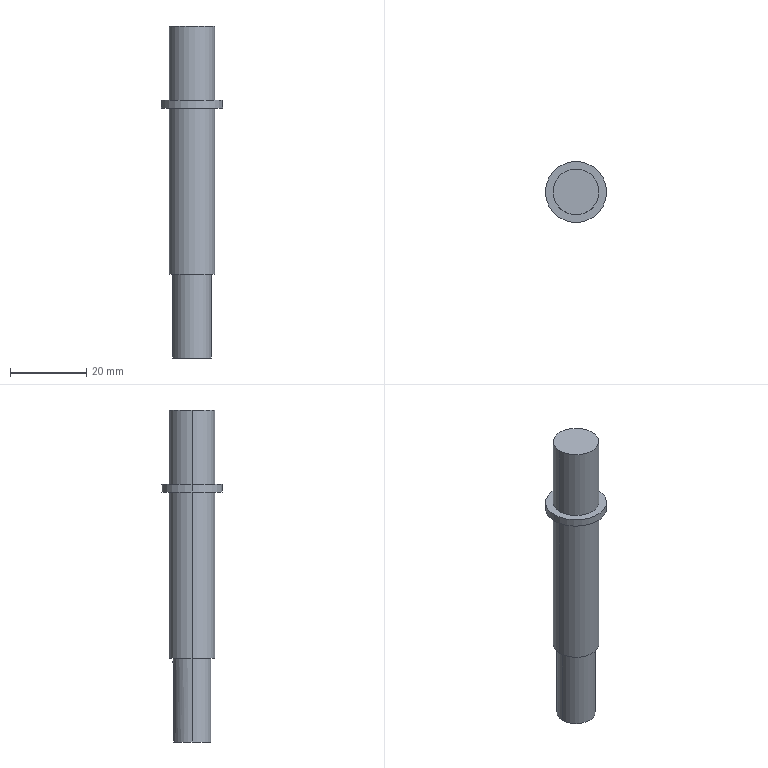Part | SolidWorks | features ICE 2, Extrusion 1, HoleWzd 1, Revolution 1 | 1 solid | 21 faces | box 16 x 16 x 87 mm | volume 9059 mm3 | cylinder 11 | plane 8 | cone 2 | commonest cylinder face diameters 12 x4 3.3 x2 10 x2 16 x2 3 x1
STEP:
#1=CARTESIAN_POINT('',(1.65,0.,-11.9));
#2=VERTEX_POINT('',#1);
#3=CARTESIAN_POINT('',(-1.65,0.,-11.9));
#4=VERTEX_POINT('',#3);
#5=CARTESIAN_POINT('',(0.,0.,-11.9));
#6=DIRECTION('',(0.,0.,-1.));
#7=DIRECTION('',(-1.,0.,0.));
#8=AXIS2_PLACEMENT_3D('',#5,#6,#7);
#9=CIRCLE('',#8,1.65);
#10=EDGE_CURVE('',#2,#4,#9,.T.);
#11=ORIENTED_EDGE('',*,*,#10,.F.);
#12=CARTESIAN_POINT('',(1.65,0.,-22.));
#13=VERTEX_POINT('',#12);
#14=CARTESIAN_POINT('',(1.65,0.,-22.));
#15=DIRECTION('',(0.,0.,-1.));
#16=VECTOR('',#15,1000.);
#17=LINE('',#14,#16);
#18=EDGE_CURVE('',#2,#13,#17,.T.);
#19=ORIENTED_EDGE('',*,*,#18,.T.);
#20=CARTESIAN_POINT('',(-1.65,0.,-22.));
#21=VERTEX_POINT('',#20);
#22=CARTESIAN_POINT('',(0.,0.,-22.));
#23=DIRECTION('',(0.,0.,-1.));
#24=DIRECTION('',(-1.,0.,0.));
#25=AXIS2_PLACEMENT_3D('',#22,#23,#24);
#26=CIRCLE('',#25,1.65);
#27=EDGE_CURVE('',#13,#21,#26,.T.);
#28=ORIENTED_EDGE('',*,*,#27,.T.);
#29=CARTESIAN_POINT('',(-1.65,0.,-22.));
#30=DIRECTION('',(0.,0.,-1.));
#31=VECTOR('',#30,1000.);
#32=LINE('',#29,#31);
#33=EDGE_CURVE('',#4,#21,#32,.T.);
#34=ORIENTED_EDGE('',*,*,#33,.F.);
#35=EDGE_LOOP('',(#11,#19,#28,#34));
#36=FACE_OUTER_BOUND('',#35,.T.);
#37=CARTESIAN_POINT('',(0.,0.,-22.));
#38=DIRECTION('',(0.,0.,-1.));
#39=DIRECTION('',(-1.,0.,0.));
#40=AXIS2_PLACEMENT_3D('',#37,#38,#39);
#41=CYLINDRICAL_SURFACE('',#40,1.65);
#42=ADVANCED_FACE('',(#36),#41,.F.);
#43=CARTESIAN_POINT('',(0.,0.,-10.909));
#44=VERTEX_POINT('',#43);
#45=CARTESIAN_POINT('',(-1.65,0.,-11.9));
#46=DIRECTION('',(-0.8572,0.,-0.515));
#47=VECTOR('',#46,1000.);
#48=LINE('',#45,#47);
#49=EDGE_CURVE('',#44,#4,#48,.T.);
#50=ORIENTED_EDGE('',*,*,#49,.F.);
#51=CARTESIAN_POINT('',(1.65,0.,-11.9));
#52=DIRECTION('',(0.8572,0.,-0.515));
#53=VECTOR('',#52,1000.);
#54=LINE('',#51,#53);
#55=EDGE_CURVE('',#44,#2,#54,.T.);
#56=ORIENTED_EDGE('',*,*,#55,.T.);
#57=ORIENTED_EDGE('',*,*,#10,.T.);
#58=EDGE_LOOP('',(#50,#56,#57));
#59=FACE_OUTER_BOUND('',#58,.T.);
#60=CARTESIAN_POINT('',(0.,0.,-11.9));
#61=DIRECTION('',(0.,0.,-1.));
#62=DIRECTION('',(-1.,0.,0.));
#63=AXIS2_PLACEMENT_3D('',#60,#61,#62);
#64=CONICAL_SURFACE('',#63,1.65,1.03);
#65=ADVANCED_FACE('',(#59),#64,.F.);
#66=CARTESIAN_POINT('',(6.,0.,65.));
#67=VERTEX_POINT('',#66);
#68=CARTESIAN_POINT('',(-6.,0.,65.));
#69=VERTEX_POINT('',#68);
#70=CARTESIAN_POINT('',(0.,0.,65.));
#71=DIRECTION('',(0.,0.,1.));
#72=DIRECTION('',(1.,0.,0.));
#73=AXIS2_PLACEMENT_3D('',#70,#71,#72);
#74=CIRCLE('',#73,6.);
#75=EDGE_CURVE('',#67,#69,#74,.T.);
#76=ORIENTED_EDGE('',*,*,#75,.F.);
#77=CARTESIAN_POINT('',(6.,0.,45.5));
#78=VERTEX_POINT('',#77);
#79=CARTESIAN_POINT('',(6.,0.,65.));
#80=DIRECTION('',(0.,0.,-1.));
#81=VECTOR('',#80,1000.);
#82=LINE('',#79,#81);
#83=EDGE_CURVE('',#67,#78,#82,.T.);
#84=ORIENTED_EDGE('',*,*,#83,.T.);
#85=CARTESIAN_POINT('',(-6.,0.,45.5));
#86=VERTEX_POINT('',#85);
#87=CARTESIAN_POINT('',(0.,0.,45.5));
#88=DIRECTION('',(0.,0.,-1.));
#89=DIRECTION('',(-1.,0.,0.));
#90=AXIS2_PLACEMENT_3D('',#87,#88,#89);
#91=CIRCLE('',#90,6.);
#92=EDGE_CURVE('',#86,#78,#91,.T.);
#93=ORIENTED_EDGE('',*,*,#92,.F.);
#94=CARTESIAN_POINT('',(-6.,0.,65.));
#95=DIRECTION('',(0.,0.,-1.));
#96=VECTOR('',#95,1000.);
#97=LINE('',#94,#96);
#98=EDGE_CURVE('',#69,#86,#97,.T.);
#99=ORIENTED_EDGE('',*,*,#98,.F.);
#100=EDGE_LOOP('',(#76,#84,#93,#99));
#101=FACE_OUTER_BOUND('',#100,.T.);
#102=CARTESIAN_POINT('',(0.,0.,65.));
#103=DIRECTION('',(0.,0.,-1.));
#104=DIRECTION('',(-1.,0.,0.));
#105=AXIS2_PLACEMENT_3D('',#102,#103,#104);
#106=CYLINDRICAL_SURFACE('',#105,6.);
#107=ADVANCED_FACE('',(#101),#106,.T.);
#108=CARTESIAN_POINT('',(8.,0.,43.5));
#109=VERTEX_POINT('',#108);
#110=CARTESIAN_POINT('',(-8.,0.,43.5));
#111=VERTEX_POINT('',#110);
#112=CARTESIAN_POINT('',(0.,0.,43.5));
#113=DIRECTION('',(0.,0.,1.));
#114=DIRECTION('',(1.,0.,0.));
#115=AXIS2_PLACEMENT_3D('',#112,#113,#114);
#116=CIRCLE('',#115,8.);
#117=EDGE_CURVE('',#109,#111,#116,.T.);
#118=ORIENTED_EDGE('',*,*,#117,.T.);
#119=CARTESIAN_POINT('',(-8.,0.,45.5));
#120=VERTEX_POINT('',#119);
#121=CARTESIAN_POINT('',(-8.,0.,65.));
#122=DIRECTION('',(0.,0.,1.));
#123=VECTOR('',#122,1000.);
#124=LINE('',#121,#123);
#125=EDGE_CURVE('',#111,#120,#124,.T.);
#126=ORIENTED_EDGE('',*,*,#125,.T.);
#127=CARTESIAN_POINT('',(8.,0.,45.5));
#128=VERTEX_POINT('',#127);
#129=CARTESIAN_POINT('',(0.,0.,45.5));
#130=DIRECTION('',(0.,0.,1.));
#131=DIRECTION('',(1.,0.,0.));
#132=AXIS2_PLACEMENT_3D('',#129,#130,#131);
#133=CIRCLE('',#132,8.);
#134=EDGE_CURVE('',#128,#120,#133,.T.);
#135=ORIENTED_EDGE('',*,*,#134,.F.);
#136=CARTESIAN_POINT('',(8.,0.,65.));
#137=DIRECTION('',(0.,0.,1.));
#138=VECTOR('',#137,1000.);
#139=LINE('',#136,#138);
#140=EDGE_CURVE('',#109,#128,#139,.T.);
#141=ORIENTED_EDGE('',*,*,#140,.F.);
#142=EDGE_LOOP('',(#118,#126,#135,#141));
#143=FACE_OUTER_BOUND('',#142,.T.);
#144=CARTESIAN_POINT('',(0.,0.,65.));
#145=DIRECTION('',(0.,0.,1.));
#146=DIRECTION('',(1.,0.,0.));
#147=AXIS2_PLACEMENT_3D('',#144,#145,#146);
#148=CYLINDRICAL_SURFACE('',#147,8.);
#149=ADVANCED_FACE('',(#143),#148,.T.);
#150=CARTESIAN_POINT('',(-5.,0.,-22.));
#151=VERTEX_POINT('',#150);
#152=CARTESIAN_POINT('',(-1.5,4.77,-22.));
#153=VERTEX_POINT('',#152);
#154=CARTESIAN_POINT('',(0.,0.,-22.));
#155=DIRECTION('',(0.,0.,-1.));
#156=DIRECTION('',(-1.,0.,0.));
#157=AXIS2_PLACEMENT_3D('',#154,#155,#156);
#158=CIRCLE('',#157,5.);
#159=EDGE_CURVE('',#151,#153,#158,.T.);
#160=ORIENTED_EDGE('',*,*,#159,.F.);
#161=CARTESIAN_POINT('',(-5.,0.,0.));
#162=VERTEX_POINT('',#161);
#163=CARTESIAN_POINT('',(-5.,0.,-22.));
#164=DIRECTION('',(0.,0.,1.));
#165=VECTOR('',#164,1000.);
#166=LINE('',#163,#165);
#167=EDGE_CURVE('',#151,#162,#166,.T.);
#168=ORIENTED_EDGE('',*,*,#167,.T.);
#169=CARTESIAN_POINT('',(5.,0.,0.));
#170=VERTEX_POINT('',#169);
#171=CARTESIAN_POINT('',(0.,0.,0.));
#172=DIRECTION('',(0.,0.,-1.));
#173=DIRECTION('',(-1.,0.,0.));
#174=AXIS2_PLACEMENT_3D('',#171,#172,#173);
#175=CIRCLE('',#174,5.);
#176=EDGE_CURVE('',#162,#170,#175,.T.);
#177=ORIENTED_EDGE('',*,*,#176,.T.);
#178=CARTESIAN_POINT('',(5.,0.,-22.));
#179=VERTEX_POINT('',#178);
#180=CARTESIAN_POINT('',(5.,0.,-22.));
#181=DIRECTION('',(0.,0.,1.));
#182=VECTOR('',#181,1000.);
#183=LINE('',#180,#182);
#184=EDGE_CURVE('',#179,#170,#183,.T.);
#185=ORIENTED_EDGE('',*,*,#184,.F.);
#186=CARTESIAN_POINT('',(1.5,4.77,-22.));
#187=VERTEX_POINT('',#186);
#188=CARTESIAN_POINT('',(0.,0.,-22.));
#189=DIRECTION('',(0.,0.,-1.));
#190=DIRECTION('',(-1.,0.,0.));
#191=AXIS2_PLACEMENT_3D('',#188,#189,#190);
#192=CIRCLE('',#191,5.);
#193=EDGE_CURVE('',#187,#179,#192,.T.);
#194=ORIENTED_EDGE('',*,*,#193,.F.);
#195=CARTESIAN_POINT('',(1.5,4.77,-2.5));
#196=VERTEX_POINT('',#195);
#197=CARTESIAN_POINT('',(1.5,4.77,-22.));
#198=DIRECTION('',(0.,0.,1.));
#199=VECTOR('',#198,1000.);
#200=LINE('',#197,#199);
#201=EDGE_CURVE('',#187,#196,#200,.T.);
#202=ORIENTED_EDGE('',*,*,#201,.T.);
#203=CARTESIAN_POINT('',(-1.5,4.77,-2.5));
#204=VERTEX_POINT('',#203);
#205=CARTESIAN_POINT('',(1.5,4.77,-2.5));
#206=CARTESIAN_POINT('',(1.5,4.77,-2.4));
#207=CARTESIAN_POINT('',(1.49,4.773,-2.302));
#208=CARTESIAN_POINT('',(1.452,4.785,-2.11));
#209=CARTESIAN_POINT('',(1.423,4.794,-2.014));
#210=CARTESIAN_POINT('',(1.347,4.815,-1.833));
#211=CARTESIAN_POINT('',(1.301,4.828,-1.747));
#212=CARTESIAN_POINT('',(1.192,4.856,-1.585));
#213=CARTESIAN_POINT('',(1.129,4.871,-1.508));
#214=CARTESIAN_POINT('',(0.9233,4.916,-1.302));
#215=CARTESIAN_POINT('',(0.7569,4.946,-1.19));
#216=CARTESIAN_POINT('',(0.3965,4.988,-1.04));
#217=CARTESIAN_POINT('',(0.1984,5.,-1.));
#218=CARTESIAN_POINT('',(-0.09698,5.,-0.9999));
#219=CARTESIAN_POINT('',(-0.197,4.997,-1.01));
#220=CARTESIAN_POINT('',(-0.3898,4.986,-1.048));
#221=CARTESIAN_POINT('',(-0.4837,4.977,-1.077));
#222=CARTESIAN_POINT('',(-0.7572,4.946,-1.19));
#223=CARTESIAN_POINT('',(-0.9219,4.916,-1.301));
#224=CARTESIAN_POINT('',(-1.13,4.871,-1.508));
#225=CARTESIAN_POINT('',(-1.191,4.856,-1.583));
#226=CARTESIAN_POINT('',(-1.3,4.828,-1.745));
#227=CARTESIAN_POINT('',(-1.347,4.815,-1.833));
#228=CARTESIAN_POINT('',(-1.46,4.783,-2.104));
#229=CARTESIAN_POINT('',(-1.5,4.77,-2.301));
#230=CARTESIAN_POINT('',(-1.5,4.77,-2.5));
#231=B_SPLINE_CURVE_WITH_KNOTS('',3,(#205,#206,#207,#208,#209,#210,#211,#212,#213,#214,#215,#216,#217,#218,#219,#220,#221,#222,#223,#224,#225,#226,#227,#228,#229,#230),.UNSPECIFIED.,.F.,.F.,(4,2,2,2,2,2,2,2,2,2,2,2,4),(0.,0.0002947,0.0005894,0.0008841,0.001179,0.001768,0.002358,0.002652,0.002947,0.003536,0.003831,0.004126,0.004715),.UNSPECIFIED.);
#232=EDGE_CURVE('',#196,#204,#231,.T.);
#233=ORIENTED_EDGE('',*,*,#232,.T.);
#234=CARTESIAN_POINT('',(-1.5,4.77,-22.));
#235=DIRECTION('',(0.,0.,-1.));
#236=VECTOR('',#235,1000.);
#237=LINE('',#234,#236);
#238=EDGE_CURVE('',#204,#153,#237,.T.);
#239=ORIENTED_EDGE('',*,*,#238,.T.);
#240=EDGE_LOOP('',(#160,#168,#177,#185,#194,#202,#233,#239));
#241=FACE_OUTER_BOUND('',#240,.T.);
#242=CARTESIAN_POINT('',(0.,0.,-22.));
#243=DIRECTION('',(0.,0.,1.));
#244=DIRECTION('',(1.,0.,0.));
#245=AXIS2_PLACEMENT_3D('',#242,#243,#244);
#246=CYLINDRICAL_SURFACE('',#245,5.);
#247=ADVANCED_FACE('',(#241),#246,.T.);
#248=CARTESIAN_POINT('',(6.,0.,43.5));
#249=VERTEX_POINT('',#248);
#250=CARTESIAN_POINT('',(-6.,0.,43.5));
#251=VERTEX_POINT('',#250);
#252=CARTESIAN_POINT('',(0.,0.,43.5));
#253=DIRECTION('',(0.,0.,1.));
#254=DIRECTION('',(1.,0.,0.));
#255=AXIS2_PLACEMENT_3D('',#252,#253,#254);
#256=CIRCLE('',#255,6.);
#257=EDGE_CURVE('',#249,#251,#256,.T.);
#258=ORIENTED_EDGE('',*,*,#257,.F.);
#259=CARTESIAN_POINT('',(6.,0.,0.));
#260=VERTEX_POINT('',#259);
#261=CARTESIAN_POINT('',(6.,0.,65.));
#262=DIRECTION('',(0.,0.,-1.));
#263=VECTOR('',#262,1000.);
#264=LINE('',#261,#263);
#265=EDGE_CURVE('',#249,#260,#264,.T.);
#266=ORIENTED_EDGE('',*,*,#265,.T.);
#267=CARTESIAN_POINT('',(-6.,0.,0.));
#268=VERTEX_POINT('',#267);
#269=CARTESIAN_POINT('',(0.,0.,0.));
#270=DIRECTION('',(0.,0.,1.));
#271=DIRECTION('',(1.,0.,0.));
#272=AXIS2_PLACEMENT_3D('',#269,#270,#271);
#273=CIRCLE('',#272,6.);
#274=EDGE_CURVE('',#260,#268,#273,.T.);
#275=ORIENTED_EDGE('',*,*,#274,.T.);
#276=CARTESIAN_POINT('',(-6.,0.,65.));
#277=DIRECTION('',(0.,0.,-1.));
#278=VECTOR('',#277,1000.);
#279=LINE('',#276,#278);
#280=EDGE_CURVE('',#251,#268,#279,.T.);
#281=ORIENTED_EDGE('',*,*,#280,.F.);
#282=EDGE_LOOP('',(#258,#266,#275,#281));
#283=FACE_OUTER_BOUND('',#282,.T.);
#284=CARTESIAN_POINT('',(0.,0.,65.));
#285=DIRECTION('',(0.,0.,-1.));
#286=DIRECTION('',(-1.,0.,0.));
#287=AXIS2_PLACEMENT_3D('',#284,#285,#286);
#288=CYLINDRICAL_SURFACE('',#287,6.);
#289=ADVANCED_FACE('',(#283),#288,.T.);
#290=ORIENTED_EDGE('',*,*,#265,.F.);
#291=CARTESIAN_POINT('',(0.,0.,43.5));
#292=DIRECTION('',(0.,0.,1.));
#293=DIRECTION('',(1.,0.,0.));
#294=AXIS2_PLACEMENT_3D('',#291,#292,#293);
#295=CIRCLE('',#294,6.);
#296=EDGE_CURVE('',#251,#249,#295,.T.);
#297=ORIENTED_EDGE('',*,*,#296,.F.);
#298=ORIENTED_EDGE('',*,*,#280,.T.);
#299=CARTESIAN_POINT('',(0.,0.,0.));
#300=DIRECTION('',(0.,0.,1.));
#301=DIRECTION('',(1.,0.,0.));
#302=AXIS2_PLACEMENT_3D('',#299,#300,#301);
#303=CIRCLE('',#302,6.);
#304=EDGE_CURVE('',#268,#260,#303,.T.);
#305=ORIENTED_EDGE('',*,*,#304,.T.);
#306=EDGE_LOOP('',(#290,#297,#298,#305));
#307=FACE_OUTER_BOUND('',#306,.T.);
#308=CARTESIAN_POINT('',(0.,0.,65.));
#309=DIRECTION('',(0.,0.,-1.));
#310=DIRECTION('',(-1.,0.,0.));
#311=AXIS2_PLACEMENT_3D('',#308,#309,#310);
#312=CYLINDRICAL_SURFACE('',#311,6.);
#313=ADVANCED_FACE('',(#307),#312,.T.);
#314=CARTESIAN_POINT('',(0.,0.,0.));
#315=DIRECTION('',(0.,0.,-1.));
#316=DIRECTION('',(-1.,0.,0.));
#317=AXIS2_PLACEMENT_3D('',#314,#315,#316);
#318=CIRCLE('',#317,5.);
#319=EDGE_CURVE('',#170,#162,#318,.T.);
#320=ORIENTED_EDGE('',*,*,#319,.F.);
#321=ORIENTED_EDGE('',*,*,#176,.F.);
#322=EDGE_LOOP('',(#320,#321));
#323=FACE_BOUND('',#322,.T.);
#324=ORIENTED_EDGE('',*,*,#304,.F.);
#325=ORIENTED_EDGE('',*,*,#274,.F.);
#326=EDGE_LOOP('',(#324,#325));
#327=FACE_OUTER_BOUND('',#326,.T.);
#328=CARTESIAN_POINT('',(0.,0.,0.));
#329=DIRECTION('',(0.,0.,1.));
#330=DIRECTION('',(1.,0.,0.));
#331=AXIS2_PLACEMENT_3D('',#328,#329,#330);
#332=PLANE('',#331);
#333=ADVANCED_FACE('',(#323,#327),#332,.F.);
#334=ORIENTED_EDGE('',*,*,#167,.F.);
#335=CARTESIAN_POINT('',(0.,0.,-22.));
#336=DIRECTION('',(0.,0.,-1.));
#337=DIRECTION('',(-1.,0.,0.));
#338=AXIS2_PLACEMENT_3D('',#335,#336,#337);
#339=CIRCLE('',#338,5.);
#340=EDGE_CURVE('',#179,#151,#339,.T.);
#341=ORIENTED_EDGE('',*,*,#340,.F.);
#342=ORIENTED_EDGE('',*,*,#184,.T.);
#343=ORIENTED_EDGE('',*,*,#319,.T.);
#344=EDGE_LOOP('',(#334,#341,#342,#343));
#345=FACE_OUTER_BOUND('',#344,.T.);
#346=CARTESIAN_POINT('',(0.,0.,-22.));
#347=DIRECTION('',(0.,0.,1.));
#348=DIRECTION('',(1.,0.,0.));
#349=AXIS2_PLACEMENT_3D('',#346,#347,#348);
#350=CYLINDRICAL_SURFACE('',#349,5.);
#351=ADVANCED_FACE('',(#345),#350,.T.);
#352=CARTESIAN_POINT('',(0.,0.,-22.));
#353=DIRECTION('',(0.,0.,-1.));
#354=DIRECTION('',(-1.,0.,0.));
#355=AXIS2_PLACEMENT_3D('',#352,#353,#354);
#356=CIRCLE('',#355,1.65);
#357=EDGE_CURVE('',#21,#13,#356,.T.);
#358=ORIENTED_EDGE('',*,*,#357,.F.);
#359=ORIENTED_EDGE('',*,*,#27,.F.);
#360=EDGE_LOOP('',(#358,#359));
#361=FACE_BOUND('',#360,.T.);
#362=CARTESIAN_POINT('',(1.5,3.2,-22.));
#363=VERTEX_POINT('',#362);
#364=CARTESIAN_POINT('',(1.5,0.,-22.));
#365=DIRECTION('',(0.,-1.,0.));
#366=VECTOR('',#365,1000.);
#367=LINE('',#364,#366);
#368=EDGE_CURVE('',#187,#363,#367,.T.);
#369=ORIENTED_EDGE('',*,*,#368,.F.);
#370=ORIENTED_EDGE('',*,*,#193,.T.);
#371=ORIENTED_EDGE('',*,*,#340,.T.);
#372=ORIENTED_EDGE('',*,*,#159,.T.);
#373=CARTESIAN_POINT('',(-1.5,3.2,-22.));
#374=VERTEX_POINT('',#373);
#375=CARTESIAN_POINT('',(-1.5,0.,-22.));
#376=DIRECTION('',(0.,1.,0.));
#377=VECTOR('',#376,1000.);
#378=LINE('',#375,#377);
#379=EDGE_CURVE('',#374,#153,#378,.T.);
#380=ORIENTED_EDGE('',*,*,#379,.F.);
#381=CARTESIAN_POINT('',(0.,3.2,-22.));
#382=DIRECTION('',(1.,0.,0.));
#383=VECTOR('',#382,1000.);
#384=LINE('',#381,#383);
#385=EDGE_CURVE('',#374,#363,#384,.T.);
#386=ORIENTED_EDGE('',*,*,#385,.T.);
#387=EDGE_LOOP('',(#369,#370,#371,#372,#380,#386));
#388=FACE_OUTER_BOUND('',#387,.T.);
#389=CARTESIAN_POINT('',(0.,0.,-22.));
#390=DIRECTION('',(0.,0.,-1.));
#391=DIRECTION('',(-1.,0.,0.));
#392=AXIS2_PLACEMENT_3D('',#389,#390,#391);
#393=PLANE('',#392);
#394=ADVANCED_FACE('',(#361,#388),#393,.T.);
#395=ORIENTED_EDGE('',*,*,#92,.T.);
#396=CARTESIAN_POINT('',(0.,0.,45.5));
#397=DIRECTION('',(0.,0.,-1.));
#398=DIRECTION('',(-1.,0.,0.));
#399=AXIS2_PLACEMENT_3D('',#396,#397,#398);
#400=CIRCLE('',#399,6.);
#401=EDGE_CURVE('',#78,#86,#400,.T.);
#402=ORIENTED_EDGE('',*,*,#401,.T.);
#403=EDGE_LOOP('',(#395,#402));
#404=FACE_BOUND('',#403,.T.);
#405=ORIENTED_EDGE('',*,*,#134,.T.);
#406=CARTESIAN_POINT('',(0.,0.,45.5));
#407=DIRECTION('',(0.,0.,1.));
#408=DIRECTION('',(1.,0.,0.));
#409=AXIS2_PLACEMENT_3D('',#406,#407,#408);
#410=CIRCLE('',#409,8.);
#411=EDGE_CURVE('',#120,#128,#410,.T.);
#412=ORIENTED_EDGE('',*,*,#411,.T.);
#413=EDGE_LOOP('',(#405,#412));
#414=FACE_OUTER_BOUND('',#413,.T.);
#415=CARTESIAN_POINT('',(-6.,0.,45.5));
#416=DIRECTION('',(0.,0.,-1.));
#417=DIRECTION('',(-1.,0.,0.));
#418=AXIS2_PLACEMENT_3D('',#415,#416,#417);
#419=PLANE('',#418);
#420=ADVANCED_FACE('',(#404,#414),#419,.F.);
#421=ORIENTED_EDGE('',*,*,#125,.F.);
#422=CARTESIAN_POINT('',(0.,0.,43.5));
#423=DIRECTION('',(0.,0.,1.));
#424=DIRECTION('',(1.,0.,0.));
#425=AXIS2_PLACEMENT_3D('',#422,#423,#424);
#426=CIRCLE('',#425,8.);
#427=EDGE_CURVE('',#111,#109,#426,.T.);
#428=ORIENTED_EDGE('',*,*,#427,.T.);
#429=ORIENTED_EDGE('',*,*,#140,.T.);
#430=ORIENTED_EDGE('',*,*,#411,.F.);
#431=EDGE_LOOP('',(#421,#428,#429,#430));
#432=FACE_OUTER_BOUND('',#431,.T.);
#433=CARTESIAN_POINT('',(0.,0.,65.));
#434=DIRECTION('',(0.,0.,1.));
#435=DIRECTION('',(1.,0.,0.));
#436=AXIS2_PLACEMENT_3D('',#433,#434,#435);
#437=CYLINDRICAL_SURFACE('',#436,8.);
#438=ADVANCED_FACE('',(#432),#437,.T.);
#439=ORIENTED_EDGE('',*,*,#117,.F.);
#440=ORIENTED_EDGE('',*,*,#427,.F.);
#441=EDGE_LOOP('',(#439,#440));
#442=FACE_OUTER_BOUND('',#441,.T.);
#443=ORIENTED_EDGE('',*,*,#296,.T.);
#444=ORIENTED_EDGE('',*,*,#257,.T.);
#445=EDGE_LOOP('',(#443,#444));
#446=FACE_BOUND('',#445,.T.);
#447=CARTESIAN_POINT('',(-6.,0.,43.5));
#448=DIRECTION('',(0.,0.,1.));
#449=DIRECTION('',(1.,0.,0.));
#450=AXIS2_PLACEMENT_3D('',#447,#448,#449);
#451=PLANE('',#450);
#452=ADVANCED_FACE('',(#442,#446),#451,.F.);
#453=CARTESIAN_POINT('',(0.,0.,65.));
#454=DIRECTION('',(0.,0.,1.));
#455=DIRECTION('',(1.,0.,0.));
#456=AXIS2_PLACEMENT_3D('',#453,#454,#455);
#457=CIRCLE('',#456,6.);
#458=EDGE_CURVE('',#69,#67,#457,.T.);
#459=ORIENTED_EDGE('',*,*,#458,.T.);
#460=ORIENTED_EDGE('',*,*,#75,.T.);
#461=EDGE_LOOP('',(#459,#460));
#462=FACE_OUTER_BOUND('',#461,.T.);
#463=CARTESIAN_POINT('',(0.,0.,65.));
#464=DIRECTION('',(0.,0.,1.));
#465=DIRECTION('',(1.,0.,0.));
#466=AXIS2_PLACEMENT_3D('',#463,#464,#465);
#467=PLANE('',#466);
#468=ADVANCED_FACE('',(#462),#467,.T.);
#469=ORIENTED_EDGE('',*,*,#83,.F.);
#470=ORIENTED_EDGE('',*,*,#458,.F.);
#471=ORIENTED_EDGE('',*,*,#98,.T.);
#472=ORIENTED_EDGE('',*,*,#401,.F.);
#473=EDGE_LOOP('',(#469,#470,#471,#472));
#474=FACE_OUTER_BOUND('',#473,.T.);
#475=CARTESIAN_POINT('',(0.,0.,65.));
#476=DIRECTION('',(0.,0.,-1.));
#477=DIRECTION('',(-1.,0.,0.));
#478=AXIS2_PLACEMENT_3D('',#475,#476,#477);
#479=CYLINDRICAL_SURFACE('',#478,6.);
#480=ADVANCED_FACE('',(#474),#479,.T.);
#481=CARTESIAN_POINT('',(1.5,3.2,-2.5));
#482=VERTEX_POINT('',#481);
#483=CARTESIAN_POINT('',(1.5,3.2,-2.5));
#484=DIRECTION('',(0.,1.,0.));
#485=VECTOR('',#484,1000.);
#486=LINE('',#483,#485);
#487=EDGE_CURVE('',#482,#196,#486,.T.);
#488=ORIENTED_EDGE('',*,*,#487,.F.);
#489=CARTESIAN_POINT('',(-1.5,3.2,-2.5));
#490=VERTEX_POINT('',#489);
#491=CARTESIAN_POINT('',(0.,3.2,-2.5));
#492=DIRECTION('',(0.,1.,0.));
#493=DIRECTION('',(-1.,0.,0.));
#494=AXIS2_PLACEMENT_3D('',#491,#492,#493);
#495=CIRCLE('',#494,1.5);
#496=EDGE_CURVE('',#490,#482,#495,.T.);
#497=ORIENTED_EDGE('',*,*,#496,.F.);
#498=CARTESIAN_POINT('',(-1.5,3.2,-2.5));
#499=DIRECTION('',(0.,1.,0.));
#500=VECTOR('',#499,1000.);
#501=LINE('',#498,#500);
#502=EDGE_CURVE('',#490,#204,#501,.T.);
#503=ORIENTED_EDGE('',*,*,#502,.T.);
#504=ORIENTED_EDGE('',*,*,#232,.F.);
#505=EDGE_LOOP('',(#488,#497,#503,#504));
#506=FACE_OUTER_BOUND('',#505,.T.);
#507=CARTESIAN_POINT('',(0.,3.2,-2.5));
#508=DIRECTION('',(0.,1.,0.));
#509=DIRECTION('',(-1.,0.,0.));
#510=AXIS2_PLACEMENT_3D('',#507,#508,#509);
#511=CYLINDRICAL_SURFACE('',#510,1.5);
#512=ADVANCED_FACE('',(#506),#511,.F.);
#513=ORIENTED_EDGE('',*,*,#368,.T.);
#514=CARTESIAN_POINT('',(1.5,3.2,-22.5));
#515=DIRECTION('',(0.,0.,-1.));
#516=VECTOR('',#515,1000.);
#517=LINE('',#514,#516);
#518=EDGE_CURVE('',#482,#363,#517,.T.);
#519=ORIENTED_EDGE('',*,*,#518,.F.);
#520=ORIENTED_EDGE('',*,*,#487,.T.);
#521=ORIENTED_EDGE('',*,*,#201,.F.);
#522=EDGE_LOOP('',(#513,#519,#520,#521));
#523=FACE_OUTER_BOUND('',#522,.T.);
#524=CARTESIAN_POINT('',(1.5,3.2,-22.5));
#525=DIRECTION('',(1.,0.,0.));
#526=DIRECTION('',(0.,1.,0.));
#527=AXIS2_PLACEMENT_3D('',#524,#525,#526);
#528=PLANE('',#527);
#529=ADVANCED_FACE('',(#523),#528,.F.);
#530=ORIENTED_EDGE('',*,*,#502,.F.);
#531=CARTESIAN_POINT('',(-1.5,3.2,-22.5));
#532=DIRECTION('',(0.,0.,1.));
#533=VECTOR('',#532,1000.);
#534=LINE('',#531,#533);
#535=EDGE_CURVE('',#374,#490,#534,.T.);
#536=ORIENTED_EDGE('',*,*,#535,.F.);
#537=ORIENTED_EDGE('',*,*,#379,.T.);
#538=ORIENTED_EDGE('',*,*,#238,.F.);
#539=EDGE_LOOP('',(#530,#536,#537,#538));
#540=FACE_OUTER_BOUND('',#539,.T.);
#541=CARTESIAN_POINT('',(-1.5,3.2,-22.5));
#542=DIRECTION('',(-1.,0.,0.));
#543=DIRECTION('',(0.,-1.,0.));
#544=AXIS2_PLACEMENT_3D('',#541,#542,#543);
#545=PLANE('',#544);
#546=ADVANCED_FACE('',(#540),#545,.F.);
#547=ORIENTED_EDGE('',*,*,#535,.T.);
#548=ORIENTED_EDGE('',*,*,#496,.T.);
#549=ORIENTED_EDGE('',*,*,#518,.T.);
#550=ORIENTED_EDGE('',*,*,#385,.F.);
#551=EDGE_LOOP('',(#547,#548,#549,#550));
#552=FACE_OUTER_BOUND('',#551,.T.);
#553=CARTESIAN_POINT('',(0.,3.2,-22.5));
#554=DIRECTION('',(0.,1.,0.));
#555=DIRECTION('',(-1.,0.,0.));
#556=AXIS2_PLACEMENT_3D('',#553,#554,#555);
#557=PLANE('',#556);
#558=ADVANCED_FACE('',(#552),#557,.T.);
#559=ORIENTED_EDGE('',*,*,#55,.F.);
#560=ORIENTED_EDGE('',*,*,#49,.T.);
#561=CARTESIAN_POINT('',(0.,0.,-11.9));
#562=DIRECTION('',(0.,0.,-1.));
#563=DIRECTION('',(-1.,0.,0.));
#564=AXIS2_PLACEMENT_3D('',#561,#562,#563);
#565=CIRCLE('',#564,1.65);
#566=EDGE_CURVE('',#4,#2,#565,.T.);
#567=ORIENTED_EDGE('',*,*,#566,.T.);
#568=EDGE_LOOP('',(#559,#560,#567));
#569=FACE_OUTER_BOUND('',#568,.T.);
#570=CARTESIAN_POINT('',(0.,0.,-11.9));
#571=DIRECTION('',(0.,0.,-1.));
#572=DIRECTION('',(-1.,0.,0.));
#573=AXIS2_PLACEMENT_3D('',#570,#571,#572);
#574=CONICAL_SURFACE('',#573,1.65,1.03);
#575=ADVANCED_FACE('',(#569),#574,.F.);
#576=ORIENTED_EDGE('',*,*,#18,.F.);
#577=ORIENTED_EDGE('',*,*,#566,.F.);
#578=ORIENTED_EDGE('',*,*,#33,.T.);
#579=ORIENTED_EDGE('',*,*,#357,.T.);
#580=EDGE_LOOP('',(#576,#577,#578,#579));
#581=FACE_OUTER_BOUND('',#580,.T.);
#582=CARTESIAN_POINT('',(0.,0.,-22.));
#583=DIRECTION('',(0.,0.,-1.));
#584=DIRECTION('',(-1.,0.,0.));
#585=AXIS2_PLACEMENT_3D('',#582,#583,#584);
#586=CYLINDRICAL_SURFACE('',#585,1.65);
#587=ADVANCED_FACE('',(#581),#586,.F.);
#588=CLOSED_SHELL('',(#42,#65,#107,#149,#247,#289,#313,#333,#351,#394,#420,#438,#452,#468,#480,#512,#529,#546,#558,#575,#587));
#589=MANIFOLD_SOLID_BREP('',#588);
#590=CARTESIAN_POINT('',(0.,0.,0.));
#591=DIRECTION('',(0.,0.,1.));
#592=DIRECTION('',(1.,0.,0.));
#593=AXIS2_PLACEMENT_3D('',#590,#591,#592);
#594=(LENGTH_UNIT()NAMED_UNIT(*)SI_UNIT(.MILLI.,.METRE.));
#595=UNCERTAINTY_MEASURE_WITH_UNIT(LENGTH_MEASURE(0.00001),#594,'','');
#596=(NAMED_UNIT(*)PLANE_ANGLE_UNIT()SI_UNIT($,.RADIAN.));
#597=(NAMED_UNIT(*)SI_UNIT($,.STERADIAN.)SOLID_ANGLE_UNIT());
#598=(GEOMETRIC_REPRESENTATION_CONTEXT(3)GLOBAL_UNCERTAINTY_ASSIGNED_CONTEXT((#595))GLOBAL_UNIT_ASSIGNED_CONTEXT((#594,#596,#597))REPRESENTATION_CONTEXT('',''));
#599=ADVANCED_BREP_SHAPE_REPRESENTATION('',(#589,#593),#598);